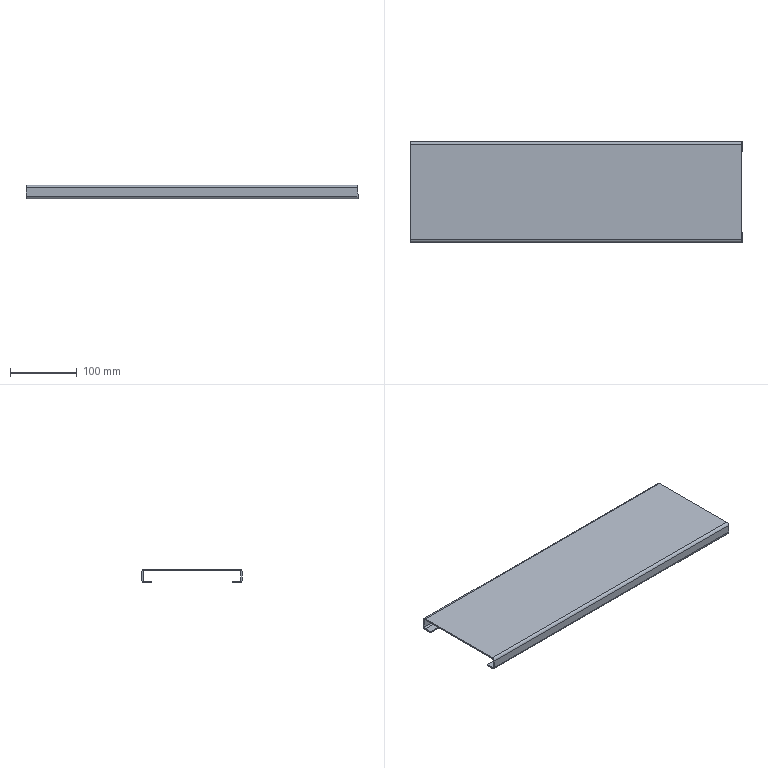Part | SolidWorks | features EdgeFlange 4, Extrusion 1, FlatPattern 1, ICE 1, SheetMetal 1, SolidToSheetMetal 1 | 1 solid | 40 faces | box 496 x 150 x 20 mm | volume 205094 mm3 | plane 30 | cylinder 10 | commonest cylinder face diameters 8 x6 4 x4
STEP:
#1=CARTESIAN_POINT('',(-233.5,73.,-13.));
#2=VERTEX_POINT('',#1);
#3=CARTESIAN_POINT('',(-233.5,73.,-5.));
#4=VERTEX_POINT('',#3);
#5=CARTESIAN_POINT('',(-233.5,73.,-9.));
#6=DIRECTION('',(0.,1.,0.));
#7=DIRECTION('',(0.,0.,1.));
#8=AXIS2_PLACEMENT_3D('',#5,#6,#7);
#9=CIRCLE('',#8,4.);
#10=EDGE_CURVE('',#2,#4,#9,.T.);
#11=ORIENTED_EDGE('',*,*,#10,.F.);
#12=CARTESIAN_POINT('',(-233.5,75.,-13.));
#13=VERTEX_POINT('',#12);
#14=CARTESIAN_POINT('',(-233.5,65.,-13.));
#15=DIRECTION('',(0.,1.,0.));
#16=VECTOR('',#15,1000.);
#17=LINE('',#14,#16);
#18=EDGE_CURVE('',#2,#13,#17,.T.);
#19=ORIENTED_EDGE('',*,*,#18,.T.);
#20=CARTESIAN_POINT('',(-233.5,75.,-5.));
#21=VERTEX_POINT('',#20);
#22=CARTESIAN_POINT('',(-233.5,75.,-9.));
#23=DIRECTION('',(0.,1.,0.));
#24=DIRECTION('',(0.,0.,1.));
#25=AXIS2_PLACEMENT_3D('',#22,#23,#24);
#26=CIRCLE('',#25,4.);
#27=EDGE_CURVE('',#13,#21,#26,.T.);
#28=ORIENTED_EDGE('',*,*,#27,.T.);
#29=CARTESIAN_POINT('',(-233.5,65.,-5.));
#30=DIRECTION('',(0.,1.,0.));
#31=VECTOR('',#30,1000.);
#32=LINE('',#29,#31);
#33=EDGE_CURVE('',#4,#21,#32,.T.);
#34=ORIENTED_EDGE('',*,*,#33,.F.);
#35=EDGE_LOOP('',(#11,#19,#28,#34));
#36=FACE_OUTER_BOUND('',#35,.T.);
#37=CARTESIAN_POINT('',(-233.5,65.,-9.));
#38=DIRECTION('',(0.,1.,0.));
#39=DIRECTION('',(0.,0.,1.));
#40=AXIS2_PLACEMENT_3D('',#37,#38,#39);
#41=CYLINDRICAL_SURFACE('',#40,4.);
#42=ADVANCED_FACE('',(#36),#41,.F.);
#43=CARTESIAN_POINT('',(-248.,-73.,-15.));
#44=VERTEX_POINT('',#43);
#45=CARTESIAN_POINT('',(-248.,-73.,-3.));
#46=VERTEX_POINT('',#45);
#47=CARTESIAN_POINT('',(-248.,-73.,-1.));
#48=DIRECTION('',(0.,0.,1.));
#49=VECTOR('',#48,1000.);
#50=LINE('',#47,#49);
#51=EDGE_CURVE('',#44,#46,#50,.T.);
#52=ORIENTED_EDGE('',*,*,#51,.F.);
#53=CARTESIAN_POINT('',(-248.,-75.,-15.));
#54=VERTEX_POINT('',#53);
#55=CARTESIAN_POINT('',(-248.,-73.,-15.));
#56=DIRECTION('',(0.,-1.,0.));
#57=VECTOR('',#56,1000.);
#58=LINE('',#55,#57);
#59=EDGE_CURVE('',#44,#54,#58,.T.);
#60=ORIENTED_EDGE('',*,*,#59,.T.);
#61=CARTESIAN_POINT('',(-248.,-75.,-3.));
#62=VERTEX_POINT('',#61);
#63=CARTESIAN_POINT('',(-248.,-75.,-1.));
#64=DIRECTION('',(0.,0.,1.));
#65=VECTOR('',#64,1000.);
#66=LINE('',#63,#65);
#67=EDGE_CURVE('',#54,#62,#66,.T.);
#68=ORIENTED_EDGE('',*,*,#67,.T.);
#69=CARTESIAN_POINT('',(-248.,-73.,-3.));
#70=DIRECTION('',(0.,-1.,0.));
#71=VECTOR('',#70,1000.);
#72=LINE('',#69,#71);
#73=EDGE_CURVE('',#46,#62,#72,.T.);
#74=ORIENTED_EDGE('',*,*,#73,.F.);
#75=EDGE_LOOP('',(#52,#60,#68,#74));
#76=FACE_OUTER_BOUND('',#75,.T.);
#77=CARTESIAN_POINT('',(-248.,-75.,-1.));
#78=DIRECTION('',(-1.,0.,0.));
#79=DIRECTION('',(0.,0.,1.));
#80=AXIS2_PLACEMENT_3D('',#77,#78,#79);
#81=PLANE('',#80);
#82=ADVANCED_FACE('',(#76),#81,.T.);
#83=ORIENTED_EDGE('',*,*,#67,.F.);
#84=CARTESIAN_POINT('',(248.,-75.,-15.));
#85=VERTEX_POINT('',#84);
#86=CARTESIAN_POINT('',(-248.,-75.,-15.));
#87=DIRECTION('',(1.,0.,0.));
#88=VECTOR('',#87,1000.);
#89=LINE('',#86,#88);
#90=EDGE_CURVE('',#54,#85,#89,.T.);
#91=ORIENTED_EDGE('',*,*,#90,.T.);
#92=CARTESIAN_POINT('',(248.,-75.,-3.));
#93=VERTEX_POINT('',#92);
#94=CARTESIAN_POINT('',(248.,-75.,-19.));
#95=DIRECTION('',(0.,0.,-1.));
#96=VECTOR('',#95,1000.);
#97=LINE('',#94,#96);
#98=EDGE_CURVE('',#93,#85,#97,.T.);
#99=ORIENTED_EDGE('',*,*,#98,.F.);
#100=CARTESIAN_POINT('',(-248.,-75.,-3.));
#101=DIRECTION('',(-1.,0.,0.));
#102=VECTOR('',#101,1000.);
#103=LINE('',#100,#102);
#104=EDGE_CURVE('',#93,#62,#103,.T.);
#105=ORIENTED_EDGE('',*,*,#104,.T.);
#106=EDGE_LOOP('',(#83,#91,#99,#105));
#107=FACE_OUTER_BOUND('',#106,.T.);
#108=CARTESIAN_POINT('',(-248.,-75.,-1.));
#109=DIRECTION('',(0.,-1.,0.));
#110=DIRECTION('',(0.,0.,-1.));
#111=AXIS2_PLACEMENT_3D('',#108,#109,#110);
#112=PLANE('',#111);
#113=ADVANCED_FACE('',(#107),#112,.T.);
#114=CARTESIAN_POINT('',(248.,-73.,-15.));
#115=VERTEX_POINT('',#114);
#116=CARTESIAN_POINT('',(-248.,-73.,-15.));
#117=DIRECTION('',(1.,0.,0.));
#118=VECTOR('',#117,1000.);
#119=LINE('',#116,#118);
#120=EDGE_CURVE('',#44,#115,#119,.T.);
#121=ORIENTED_EDGE('',*,*,#120,.F.);
#122=ORIENTED_EDGE('',*,*,#51,.T.);
#123=CARTESIAN_POINT('',(248.,-73.,-3.));
#124=VERTEX_POINT('',#123);
#125=CARTESIAN_POINT('',(248.,-73.,-3.));
#126=DIRECTION('',(-1.,0.,0.));
#127=VECTOR('',#126,1000.);
#128=LINE('',#125,#127);
#129=EDGE_CURVE('',#124,#46,#128,.T.);
#130=ORIENTED_EDGE('',*,*,#129,.F.);
#131=CARTESIAN_POINT('',(248.,-73.,-1.));
#132=DIRECTION('',(0.,0.,-1.));
#133=VECTOR('',#132,1000.);
#134=LINE('',#131,#133);
#135=EDGE_CURVE('',#124,#115,#134,.T.);
#136=ORIENTED_EDGE('',*,*,#135,.T.);
#137=EDGE_LOOP('',(#121,#122,#130,#136));
#138=FACE_OUTER_BOUND('',#137,.T.);
#139=CARTESIAN_POINT('',(-248.,-73.,-1.));
#140=DIRECTION('',(0.,-1.,0.));
#141=DIRECTION('',(0.,0.,-1.));
#142=AXIS2_PLACEMENT_3D('',#139,#140,#141);
#143=PLANE('',#142);
#144=ADVANCED_FACE('',(#138),#143,.F.);
#145=CARTESIAN_POINT('',(-248.,71.,1.));
#146=VERTEX_POINT('',#145);
#147=CARTESIAN_POINT('',(-248.,-71.,1.));
#148=VERTEX_POINT('',#147);
#149=CARTESIAN_POINT('',(-248.,75.,1.));
#150=DIRECTION('',(0.,-1.,0.));
#151=VECTOR('',#150,1000.);
#152=LINE('',#149,#151);
#153=EDGE_CURVE('',#146,#148,#152,.T.);
#154=ORIENTED_EDGE('',*,*,#153,.T.);
#155=CARTESIAN_POINT('',(248.,-71.,1.));
#156=VERTEX_POINT('',#155);
#157=CARTESIAN_POINT('',(-248.,-71.,1.));
#158=DIRECTION('',(1.,0.,0.));
#159=VECTOR('',#158,1000.);
#160=LINE('',#157,#159);
#161=EDGE_CURVE('',#148,#156,#160,.T.);
#162=ORIENTED_EDGE('',*,*,#161,.T.);
#163=CARTESIAN_POINT('',(248.,71.,1.));
#164=VERTEX_POINT('',#163);
#165=CARTESIAN_POINT('',(248.,75.,1.));
#166=DIRECTION('',(0.,1.,0.));
#167=VECTOR('',#166,1000.);
#168=LINE('',#165,#167);
#169=EDGE_CURVE('',#156,#164,#168,.T.);
#170=ORIENTED_EDGE('',*,*,#169,.T.);
#171=CARTESIAN_POINT('',(248.,71.,1.));
#172=DIRECTION('',(-1.,0.,0.));
#173=VECTOR('',#172,1000.);
#174=LINE('',#171,#173);
#175=EDGE_CURVE('',#164,#146,#174,.T.);
#176=ORIENTED_EDGE('',*,*,#175,.T.);
#177=EDGE_LOOP('',(#154,#162,#170,#176));
#178=FACE_OUTER_BOUND('',#177,.T.);
#179=CARTESIAN_POINT('',(248.,-75.,1.));
#180=DIRECTION('',(0.,0.,1.));
#181=DIRECTION('',(1.,0.,0.));
#182=AXIS2_PLACEMENT_3D('',#179,#180,#181);
#183=PLANE('',#182);
#184=ADVANCED_FACE('',(#178),#183,.T.);
#185=CARTESIAN_POINT('',(-248.,-71.,-1.));
#186=VERTEX_POINT('',#185);
#187=CARTESIAN_POINT('',(248.,-71.,-1.));
#188=VERTEX_POINT('',#187);
#189=CARTESIAN_POINT('',(-248.,-71.,-1.));
#190=DIRECTION('',(1.,0.,0.));
#191=VECTOR('',#190,1000.);
#192=LINE('',#189,#191);
#193=EDGE_CURVE('',#186,#188,#192,.T.);
#194=ORIENTED_EDGE('',*,*,#193,.F.);
#195=CARTESIAN_POINT('',(-248.,71.,-1.));
#196=VERTEX_POINT('',#195);
#197=CARTESIAN_POINT('',(-248.,-75.,-1.));
#198=DIRECTION('',(0.,-1.,0.));
#199=VECTOR('',#198,1000.);
#200=LINE('',#197,#199);
#201=EDGE_CURVE('',#196,#186,#200,.T.);
#202=ORIENTED_EDGE('',*,*,#201,.F.);
#203=CARTESIAN_POINT('',(248.,71.,-1.));
#204=VERTEX_POINT('',#203);
#205=CARTESIAN_POINT('',(248.,71.,-1.));
#206=DIRECTION('',(-1.,0.,0.));
#207=VECTOR('',#206,1000.);
#208=LINE('',#205,#207);
#209=EDGE_CURVE('',#204,#196,#208,.T.);
#210=ORIENTED_EDGE('',*,*,#209,.F.);
#211=CARTESIAN_POINT('',(248.,-75.,-1.));
#212=DIRECTION('',(0.,1.,0.));
#213=VECTOR('',#212,1000.);
#214=LINE('',#211,#213);
#215=EDGE_CURVE('',#188,#204,#214,.T.);
#216=ORIENTED_EDGE('',*,*,#215,.F.);
#217=EDGE_LOOP('',(#194,#202,#210,#216));
#218=FACE_OUTER_BOUND('',#217,.T.);
#219=CARTESIAN_POINT('',(248.,-75.,-1.));
#220=DIRECTION('',(0.,0.,1.));
#221=DIRECTION('',(1.,0.,0.));
#222=AXIS2_PLACEMENT_3D('',#219,#220,#221);
#223=PLANE('',#222);
#224=ADVANCED_FACE('',(#218),#223,.F.);
#225=ORIENTED_EDGE('',*,*,#201,.T.);
#226=CARTESIAN_POINT('',(-248.,-71.,-1.));
#227=DIRECTION('',(0.,0.,1.));
#228=VECTOR('',#227,1000.);
#229=LINE('',#226,#228);
#230=EDGE_CURVE('',#186,#148,#229,.T.);
#231=ORIENTED_EDGE('',*,*,#230,.T.);
#232=ORIENTED_EDGE('',*,*,#153,.F.);
#233=CARTESIAN_POINT('',(-248.,71.,-1.));
#234=DIRECTION('',(0.,0.,1.));
#235=VECTOR('',#234,1000.);
#236=LINE('',#233,#235);
#237=EDGE_CURVE('',#196,#146,#236,.T.);
#238=ORIENTED_EDGE('',*,*,#237,.F.);
#239=EDGE_LOOP('',(#225,#231,#232,#238));
#240=FACE_OUTER_BOUND('',#239,.T.);
#241=CARTESIAN_POINT('',(-248.,75.,1.));
#242=DIRECTION('',(-1.,0.,0.));
#243=DIRECTION('',(0.,-1.,0.));
#244=AXIS2_PLACEMENT_3D('',#241,#242,#243);
#245=PLANE('',#244);
#246=ADVANCED_FACE('',(#240),#245,.T.);
#247=CARTESIAN_POINT('',(248.,73.,-15.));
#248=VERTEX_POINT('',#247);
#249=CARTESIAN_POINT('',(248.,73.,-3.));
#250=VERTEX_POINT('',#249);
#251=CARTESIAN_POINT('',(248.,73.,-1.));
#252=DIRECTION('',(0.,0.,1.));
#253=VECTOR('',#252,1000.);
#254=LINE('',#251,#253);
#255=EDGE_CURVE('',#248,#250,#254,.T.);
#256=ORIENTED_EDGE('',*,*,#255,.F.);
#257=CARTESIAN_POINT('',(248.,75.,-15.));
#258=VERTEX_POINT('',#257);
#259=CARTESIAN_POINT('',(248.,73.,-15.));
#260=DIRECTION('',(0.,1.,0.));
#261=VECTOR('',#260,1000.);
#262=LINE('',#259,#261);
#263=EDGE_CURVE('',#248,#258,#262,.T.);
#264=ORIENTED_EDGE('',*,*,#263,.T.);
#265=CARTESIAN_POINT('',(248.,75.,-3.));
#266=VERTEX_POINT('',#265);
#267=CARTESIAN_POINT('',(248.,75.,-1.));
#268=DIRECTION('',(0.,0.,1.));
#269=VECTOR('',#268,1000.);
#270=LINE('',#267,#269);
#271=EDGE_CURVE('',#258,#266,#270,.T.);
#272=ORIENTED_EDGE('',*,*,#271,.T.);
#273=CARTESIAN_POINT('',(248.,73.,-3.));
#274=DIRECTION('',(0.,1.,0.));
#275=VECTOR('',#274,1000.);
#276=LINE('',#273,#275);
#277=EDGE_CURVE('',#250,#266,#276,.T.);
#278=ORIENTED_EDGE('',*,*,#277,.F.);
#279=EDGE_LOOP('',(#256,#264,#272,#278));
#280=FACE_OUTER_BOUND('',#279,.T.);
#281=CARTESIAN_POINT('',(248.,75.,-1.));
#282=DIRECTION('',(1.,0.,0.));
#283=DIRECTION('',(0.,0.,-1.));
#284=AXIS2_PLACEMENT_3D('',#281,#282,#283);
#285=PLANE('',#284);
#286=ADVANCED_FACE('',(#280),#285,.T.);
#287=CARTESIAN_POINT('',(-233.5,75.,-9.));
#288=DIRECTION('',(0.,1.,0.));
#289=DIRECTION('',(0.,0.,1.));
#290=AXIS2_PLACEMENT_3D('',#287,#288,#289);
#291=CIRCLE('',#290,4.);
#292=EDGE_CURVE('',#21,#13,#291,.T.);
#293=ORIENTED_EDGE('',*,*,#292,.F.);
#294=ORIENTED_EDGE('',*,*,#27,.F.);
#295=EDGE_LOOP('',(#293,#294));
#296=FACE_BOUND('',#295,.T.);
#297=ORIENTED_EDGE('',*,*,#271,.F.);
#298=CARTESIAN_POINT('',(-248.,75.,-15.));
#299=VERTEX_POINT('',#298);
#300=CARTESIAN_POINT('',(248.,75.,-15.));
#301=DIRECTION('',(-1.,0.,0.));
#302=VECTOR('',#301,1000.);
#303=LINE('',#300,#302);
#304=EDGE_CURVE('',#258,#299,#303,.T.);
#305=ORIENTED_EDGE('',*,*,#304,.T.);
#306=CARTESIAN_POINT('',(-248.,75.,-3.));
#307=VERTEX_POINT('',#306);
#308=CARTESIAN_POINT('',(-248.,75.,-19.));
#309=DIRECTION('',(0.,0.,-1.));
#310=VECTOR('',#309,1000.);
#311=LINE('',#308,#310);
#312=EDGE_CURVE('',#307,#299,#311,.T.);
#313=ORIENTED_EDGE('',*,*,#312,.F.);
#314=CARTESIAN_POINT('',(248.,75.,-3.));
#315=DIRECTION('',(1.,0.,0.));
#316=VECTOR('',#315,1000.);
#317=LINE('',#314,#316);
#318=EDGE_CURVE('',#307,#266,#317,.T.);
#319=ORIENTED_EDGE('',*,*,#318,.T.);
#320=EDGE_LOOP('',(#297,#305,#313,#319));
#321=FACE_OUTER_BOUND('',#320,.T.);
#322=CARTESIAN_POINT('',(248.,75.,-1.));
#323=DIRECTION('',(0.,1.,0.));
#324=DIRECTION('',(0.,0.,1.));
#325=AXIS2_PLACEMENT_3D('',#322,#323,#324);
#326=PLANE('',#325);
#327=ADVANCED_FACE('',(#296,#321),#326,.T.);
#328=CARTESIAN_POINT('',(-233.5,73.,-9.));
#329=DIRECTION('',(0.,1.,0.));
#330=DIRECTION('',(0.,0.,1.));
#331=AXIS2_PLACEMENT_3D('',#328,#329,#330);
#332=CIRCLE('',#331,4.);
#333=EDGE_CURVE('',#4,#2,#332,.T.);
#334=ORIENTED_EDGE('',*,*,#333,.T.);
#335=ORIENTED_EDGE('',*,*,#10,.T.);
#336=EDGE_LOOP('',(#334,#335));
#337=FACE_BOUND('',#336,.T.);
#338=CARTESIAN_POINT('',(-248.,73.,-15.));
#339=VERTEX_POINT('',#338);
#340=CARTESIAN_POINT('',(248.,73.,-15.));
#341=DIRECTION('',(-1.,0.,0.));
#342=VECTOR('',#341,1000.);
#343=LINE('',#340,#342);
#344=EDGE_CURVE('',#248,#339,#343,.T.);
#345=ORIENTED_EDGE('',*,*,#344,.F.);
#346=ORIENTED_EDGE('',*,*,#255,.T.);
#347=CARTESIAN_POINT('',(-248.,73.,-3.));
#348=VERTEX_POINT('',#347);
#349=CARTESIAN_POINT('',(-248.,73.,-3.));
#350=DIRECTION('',(1.,0.,0.));
#351=VECTOR('',#350,1000.);
#352=LINE('',#349,#351);
#353=EDGE_CURVE('',#348,#250,#352,.T.);
#354=ORIENTED_EDGE('',*,*,#353,.F.);
#355=CARTESIAN_POINT('',(-248.,73.,-1.));
#356=DIRECTION('',(0.,0.,-1.));
#357=VECTOR('',#356,1000.);
#358=LINE('',#355,#357);
#359=EDGE_CURVE('',#348,#339,#358,.T.);
#360=ORIENTED_EDGE('',*,*,#359,.T.);
#361=EDGE_LOOP('',(#345,#346,#354,#360));
#362=FACE_OUTER_BOUND('',#361,.T.);
#363=CARTESIAN_POINT('',(248.,73.,-1.));
#364=DIRECTION('',(0.,1.,0.));
#365=DIRECTION('',(0.,0.,1.));
#366=AXIS2_PLACEMENT_3D('',#363,#364,#365);
#367=PLANE('',#366);
#368=ADVANCED_FACE('',(#337,#362),#367,.F.);
#369=CARTESIAN_POINT('',(248.,-71.,-1.));
#370=DIRECTION('',(0.,0.,1.));
#371=VECTOR('',#370,1000.);
#372=LINE('',#369,#371);
#373=EDGE_CURVE('',#188,#156,#372,.T.);
#374=ORIENTED_EDGE('',*,*,#373,.F.);
#375=ORIENTED_EDGE('',*,*,#215,.T.);
#376=CARTESIAN_POINT('',(248.,71.,-1.));
#377=DIRECTION('',(0.,0.,1.));
#378=VECTOR('',#377,1000.);
#379=LINE('',#376,#378);
#380=EDGE_CURVE('',#204,#164,#379,.T.);
#381=ORIENTED_EDGE('',*,*,#380,.T.);
#382=ORIENTED_EDGE('',*,*,#169,.F.);
#383=EDGE_LOOP('',(#374,#375,#381,#382));
#384=FACE_OUTER_BOUND('',#383,.T.);
#385=CARTESIAN_POINT('',(248.,75.,1.));
#386=DIRECTION('',(1.,0.,0.));
#387=DIRECTION('',(0.,1.,0.));
#388=AXIS2_PLACEMENT_3D('',#385,#386,#387);
#389=PLANE('',#388);
#390=ADVANCED_FACE('',(#384),#389,.T.);
#391=CARTESIAN_POINT('',(-248.,75.,-3.));
#392=DIRECTION('',(0.,1.,0.));
#393=VECTOR('',#392,1000.);
#394=LINE('',#391,#393);
#395=EDGE_CURVE('',#348,#307,#394,.T.);
#396=ORIENTED_EDGE('',*,*,#395,.F.);
#397=CARTESIAN_POINT('',(-248.,71.,-3.));
#398=DIRECTION('',(-1.,0.,0.));
#399=DIRECTION('',(0.,0.,-1.));
#400=AXIS2_PLACEMENT_3D('',#397,#398,#399);
#401=CIRCLE('',#400,2.);
#402=EDGE_CURVE('',#196,#348,#401,.T.);
#403=ORIENTED_EDGE('',*,*,#402,.F.);
#404=ORIENTED_EDGE('',*,*,#237,.T.);
#405=CARTESIAN_POINT('',(-248.,71.,-3.));
#406=DIRECTION('',(-1.,0.,0.));
#407=DIRECTION('',(0.,0.,-1.));
#408=AXIS2_PLACEMENT_3D('',#405,#406,#407);
#409=CIRCLE('',#408,4.);
#410=EDGE_CURVE('',#146,#307,#409,.T.);
#411=ORIENTED_EDGE('',*,*,#410,.T.);
#412=EDGE_LOOP('',(#396,#403,#404,#411));
#413=FACE_OUTER_BOUND('',#412,.T.);
#414=CARTESIAN_POINT('',(-248.,71.,-3.));
#415=DIRECTION('',(-1.,0.,0.));
#416=DIRECTION('',(0.,0.,1.));
#417=AXIS2_PLACEMENT_3D('',#414,#415,#416);
#418=PLANE('',#417);
#419=ADVANCED_FACE('',(#413),#418,.T.);
#420=ORIENTED_EDGE('',*,*,#175,.F.);
#421=CARTESIAN_POINT('',(248.,71.,-3.));
#422=DIRECTION('',(1.,0.,0.));
#423=DIRECTION('',(0.,0.,-1.));
#424=AXIS2_PLACEMENT_3D('',#421,#422,#423);
#425=CIRCLE('',#424,4.);
#426=EDGE_CURVE('',#266,#164,#425,.T.);
#427=ORIENTED_EDGE('',*,*,#426,.F.);
#428=ORIENTED_EDGE('',*,*,#318,.F.);
#429=ORIENTED_EDGE('',*,*,#410,.F.);
#430=EDGE_LOOP('',(#420,#427,#428,#429));
#431=FACE_OUTER_BOUND('',#430,.T.);
#432=CARTESIAN_POINT('',(248.,71.,-3.));
#433=DIRECTION('',(1.,0.,0.));
#434=DIRECTION('',(0.,1.,0.));
#435=AXIS2_PLACEMENT_3D('',#432,#433,#434);
#436=CYLINDRICAL_SURFACE('',#435,4.);
#437=ADVANCED_FACE('',(#431),#436,.T.);
#438=CARTESIAN_POINT('',(248.,71.,-3.));
#439=DIRECTION('',(1.,0.,0.));
#440=DIRECTION('',(0.,0.,-1.));
#441=AXIS2_PLACEMENT_3D('',#438,#439,#440);
#442=CIRCLE('',#441,2.);
#443=EDGE_CURVE('',#250,#204,#442,.T.);
#444=ORIENTED_EDGE('',*,*,#443,.F.);
#445=ORIENTED_EDGE('',*,*,#277,.T.);
#446=ORIENTED_EDGE('',*,*,#426,.T.);
#447=ORIENTED_EDGE('',*,*,#380,.F.);
#448=EDGE_LOOP('',(#444,#445,#446,#447));
#449=FACE_OUTER_BOUND('',#448,.T.);
#450=CARTESIAN_POINT('',(248.,71.,-3.));
#451=DIRECTION('',(-1.,0.,0.));
#452=DIRECTION('',(0.,0.,1.));
#453=AXIS2_PLACEMENT_3D('',#450,#451,#452);
#454=PLANE('',#453);
#455=ADVANCED_FACE('',(#449),#454,.F.);
#456=ORIENTED_EDGE('',*,*,#209,.T.);
#457=ORIENTED_EDGE('',*,*,#402,.T.);
#458=ORIENTED_EDGE('',*,*,#353,.T.);
#459=ORIENTED_EDGE('',*,*,#443,.T.);
#460=EDGE_LOOP('',(#456,#457,#458,#459));
#461=FACE_OUTER_BOUND('',#460,.T.);
#462=CARTESIAN_POINT('',(248.,71.,-3.));
#463=DIRECTION('',(1.,0.,0.));
#464=DIRECTION('',(0.,1.,0.));
#465=AXIS2_PLACEMENT_3D('',#462,#463,#464);
#466=CYLINDRICAL_SURFACE('',#465,2.);
#467=ADVANCED_FACE('',(#461),#466,.F.);
#468=CARTESIAN_POINT('',(-248.,73.,-15.));
#469=DIRECTION('',(0.,1.,0.));
#470=VECTOR('',#469,1000.);
#471=LINE('',#468,#470);
#472=EDGE_CURVE('',#339,#299,#471,.T.);
#473=ORIENTED_EDGE('',*,*,#472,.F.);
#474=ORIENTED_EDGE('',*,*,#359,.F.);
#475=ORIENTED_EDGE('',*,*,#395,.T.);
#476=ORIENTED_EDGE('',*,*,#312,.T.);
#477=EDGE_LOOP('',(#473,#474,#475,#476));
#478=FACE_OUTER_BOUND('',#477,.T.);
#479=CARTESIAN_POINT('',(-248.,75.,-19.));
#480=DIRECTION('',(-1.,0.,0.));
#481=DIRECTION('',(0.,0.,1.));
#482=AXIS2_PLACEMENT_3D('',#479,#480,#481);
#483=PLANE('',#482);
#484=ADVANCED_FACE('',(#478),#483,.T.);
#485=CARTESIAN_POINT('',(-248.,71.,-17.));
#486=VERTEX_POINT('',#485);
#487=CARTESIAN_POINT('',(-248.,71.,-19.));
#488=VERTEX_POINT('',#487);
#489=CARTESIAN_POINT('',(-248.,71.,-19.));
#490=DIRECTION('',(0.,0.,-1.));
#491=VECTOR('',#490,1000.);
#492=LINE('',#489,#491);
#493=EDGE_CURVE('',#486,#488,#492,.T.);
#494=ORIENTED_EDGE('',*,*,#493,.F.);
#495=CARTESIAN_POINT('',(-248.,71.,-15.));
#496=DIRECTION('',(-1.,0.,0.));
#497=DIRECTION('',(0.,0.,-1.));
#498=AXIS2_PLACEMENT_3D('',#495,#496,#497);
#499=CIRCLE('',#498,2.);
#500=EDGE_CURVE('',#339,#486,#499,.T.);
#501=ORIENTED_EDGE('',*,*,#500,.F.);
#502=ORIENTED_EDGE('',*,*,#472,.T.);
#503=CARTESIAN_POINT('',(-248.,71.,-15.));
#504=DIRECTION('',(-1.,0.,0.));
#505=DIRECTION('',(0.,0.,-1.));
#506=AXIS2_PLACEMENT_3D('',#503,#504,#505);
#507=CIRCLE('',#506,4.);
#508=EDGE_CURVE('',#299,#488,#507,.T.);
#509=ORIENTED_EDGE('',*,*,#508,.T.);
#510=EDGE_LOOP('',(#494,#501,#502,#509));
#511=FACE_OUTER_BOUND('',#510,.T.);
#512=CARTESIAN_POINT('',(-248.,71.,-15.));
#513=DIRECTION('',(-1.,0.,0.));
#514=DIRECTION('',(0.,0.,1.));
#515=AXIS2_PLACEMENT_3D('',#512,#513,#514);
#516=PLANE('',#515);
#517=ADVANCED_FACE('',(#511),#516,.T.);
#518=ORIENTED_EDGE('',*,*,#304,.F.);
#519=CARTESIAN_POINT('',(248.,71.,-19.));
#520=VERTEX_POINT('',#519);
#521=CARTESIAN_POINT('',(248.,71.,-15.));
#522=DIRECTION('',(1.,0.,0.));
#523=DIRECTION('',(0.,0.,-1.));
#524=AXIS2_PLACEMENT_3D('',#521,#522,#523);
#525=CIRCLE('',#524,4.);
#526=EDGE_CURVE('',#520,#258,#525,.T.);
#527=ORIENTED_EDGE('',*,*,#526,.F.);
#528=CARTESIAN_POINT('',(248.,71.,-19.));
#529=DIRECTION('',(1.,0.,0.));
#530=VECTOR('',#529,1000.);
#531=LINE('',#528,#530);
#532=EDGE_CURVE('',#488,#520,#531,.T.);
#533=ORIENTED_EDGE('',*,*,#532,.F.);
#534=ORIENTED_EDGE('',*,*,#508,.F.);
#535=EDGE_LOOP('',(#518,#527,#533,#534));
#536=FACE_OUTER_BOUND('',#535,.T.);
#537=CARTESIAN_POINT('',(248.,71.,-15.));
#538=DIRECTION('',(1.,0.,0.));
#539=DIRECTION('',(0.,0.,-1.));
#540=AXIS2_PLACEMENT_3D('',#537,#538,#539);
#541=CYLINDRICAL_SURFACE('',#540,4.);
#542=ADVANCED_FACE('',(#536),#541,.T.);
#543=CARTESIAN_POINT('',(248.,71.,-17.));
#544=VERTEX_POINT('',#543);
#545=CARTESIAN_POINT('',(248.,71.,-15.));
#546=DIRECTION('',(1.,0.,0.));
#547=DIRECTION('',(0.,0.,-1.));
#548=AXIS2_PLACEMENT_3D('',#545,#546,#547);
#549=CIRCLE('',#548,2.);
#550=EDGE_CURVE('',#544,#248,#549,.T.);
#551=ORIENTED_EDGE('',*,*,#550,.F.);
#552=CARTESIAN_POINT('',(248.,71.,-17.));
#553=DIRECTION('',(0.,0.,-1.));
#554=VECTOR('',#553,1000.);
#555=LINE('',#552,#554);
#556=EDGE_CURVE('',#544,#520,#555,.T.);
#557=ORIENTED_EDGE('',*,*,#556,.T.);
#558=ORIENTED_EDGE('',*,*,#526,.T.);
#559=ORIENTED_EDGE('',*,*,#263,.F.);
#560=EDGE_LOOP('',(#551,#557,#558,#559));
#561=FACE_OUTER_BOUND('',#560,.T.);
#562=CARTESIAN_POINT('',(248.,71.,-15.));
#563=DIRECTION('',(-1.,0.,0.));
#564=DIRECTION('',(0.,0.,1.));
#565=AXIS2_PLACEMENT_3D('',#562,#563,#564);
#566=PLANE('',#565);
#567=ADVANCED_FACE('',(#561),#566,.F.);
#568=ORIENTED_EDGE('',*,*,#344,.T.);
#569=ORIENTED_EDGE('',*,*,#500,.T.);
#570=CARTESIAN_POINT('',(-248.,71.,-17.));
#571=DIRECTION('',(1.,0.,0.));
#572=VECTOR('',#571,1000.);
#573=LINE('',#570,#572);
#574=EDGE_CURVE('',#486,#544,#573,.T.);
#575=ORIENTED_EDGE('',*,*,#574,.T.);
#576=ORIENTED_EDGE('',*,*,#550,.T.);
#577=EDGE_LOOP('',(#568,#569,#575,#576));
#578=FACE_OUTER_BOUND('',#577,.T.);
#579=CARTESIAN_POINT('',(248.,71.,-15.));
#580=DIRECTION('',(1.,0.,0.));
#581=DIRECTION('',(0.,0.,-1.));
#582=AXIS2_PLACEMENT_3D('',#579,#580,#581);
#583=CYLINDRICAL_SURFACE('',#582,2.);
#584=ADVANCED_FACE('',(#578),#583,.F.);
#585=CARTESIAN_POINT('',(248.,60.,-19.));
#586=VERTEX_POINT('',#585);
#587=CARTESIAN_POINT('',(248.,73.,-19.));
#588=DIRECTION('',(0.,1.,0.));
#589=VECTOR('',#588,1000.);
#590=LINE('',#587,#589);
#591=EDGE_CURVE('',#586,#520,#590,.T.);
#592=ORIENTED_EDGE('',*,*,#591,.T.);
#593=ORIENTED_EDGE('',*,*,#556,.F.);
#594=CARTESIAN_POINT('',(248.,60.,-17.));
#595=VERTEX_POINT('',#594);
#596=CARTESIAN_POINT('',(248.,73.,-17.));
#597=DIRECTION('',(0.,1.,0.));
#598=VECTOR('',#597,1000.);
#599=LINE('',#596,#598);
#600=EDGE_CURVE('',#595,#544,#599,.T.);
#601=ORIENTED_EDGE('',*,*,#600,.F.);
#602=CARTESIAN_POINT('',(248.,60.,-19.));
#603=DIRECTION('',(0.,0.,1.));
#604=VECTOR('',#603,1000.);
#605=LINE('',#602,#604);
#606=EDGE_CURVE('',#586,#595,#605,.T.);
#607=ORIENTED_EDGE('',*,*,#606,.F.);
#608=EDGE_LOOP('',(#592,#593,#601,#607));
#609=FACE_OUTER_BOUND('',#608,.T.);
#610=CARTESIAN_POINT('',(248.,73.,-19.));
#611=DIRECTION('',(1.,0.,0.));
#612=DIRECTION('',(0.,0.,-1.));
#613=AXIS2_PLACEMENT_3D('',#610,#611,#612);
#614=PLANE('',#613);
#615=ADVANCED_FACE('',(#609),#614,.T.);
#616=CARTESIAN_POINT('',(-248.,60.,-17.));
#617=VERTEX_POINT('',#616);
#618=CARTESIAN_POINT('',(-248.,73.,-17.));
#619=DIRECTION('',(0.,-1.,0.));
#620=VECTOR('',#619,1000.);
#621=LINE('',#618,#620);
#622=EDGE_CURVE('',#486,#617,#621,.T.);
#623=ORIENTED_EDGE('',*,*,#622,.F.);
#624=ORIENTED_EDGE('',*,*,#493,.T.);
#625=CARTESIAN_POINT('',(-248.,60.,-19.));
#626=VERTEX_POINT('',#625);
#627=CARTESIAN_POINT('',(-248.,60.,-19.));
#628=DIRECTION('',(0.,-1.,0.));
#629=VECTOR('',#628,1000.);
#630=LINE('',#627,#629);
#631=EDGE_CURVE('',#488,#626,#630,.T.);
#632=ORIENTED_EDGE('',*,*,#631,.T.);
#633=CARTESIAN_POINT('',(-248.,60.,-19.));
#634=DIRECTION('',(0.,0.,1.));
#635=VECTOR('',#634,1000.);
#636=LINE('',#633,#635);
#637=EDGE_CURVE('',#626,#617,#636,.T.);
#638=ORIENTED_EDGE('',*,*,#637,.T.);
#639=EDGE_LOOP('',(#623,#624,#632,#638));
#640=FACE_OUTER_BOUND('',#639,.T.);
#641=CARTESIAN_POINT('',(-248.,60.,-19.));
#642=DIRECTION('',(-1.,0.,0.));
#643=DIRECTION('',(0.,0.,1.));
#644=AXIS2_PLACEMENT_3D('',#641,#642,#643);
#645=PLANE('',#644);
#646=ADVANCED_FACE('',(#640),#645,.T.);
#647=ORIENTED_EDGE('',*,*,#631,.F.);
#648=ORIENTED_EDGE('',*,*,#532,.T.);
#649=ORIENTED_EDGE('',*,*,#591,.F.);
#650=CARTESIAN_POINT('',(248.,60.,-19.));
#651=DIRECTION('',(1.,0.,0.));
#652=VECTOR('',#651,1000.);
#653=LINE('',#650,#652);
#654=EDGE_CURVE('',#626,#586,#653,.T.);
#655=ORIENTED_EDGE('',*,*,#654,.F.);
#656=EDGE_LOOP('',(#647,#648,#649,#655));
#657=FACE_OUTER_BOUND('',#656,.T.);
#658=CARTESIAN_POINT('',(248.,73.,-19.));
#659=DIRECTION('',(0.,0.,-1.));
#660=DIRECTION('',(0.,1.,0.));
#661=AXIS2_PLACEMENT_3D('',#658,#659,#660);
#662=PLANE('',#661);
#663=ADVANCED_FACE('',(#657),#662,.T.);
#664=ORIENTED_EDGE('',*,*,#574,.F.);
#665=ORIENTED_EDGE('',*,*,#622,.T.);
#666=CARTESIAN_POINT('',(248.,60.,-17.));
#667=DIRECTION('',(1.,0.,0.));
#668=VECTOR('',#667,1000.);
#669=LINE('',#666,#668);
#670=EDGE_CURVE('',#617,#595,#669,.T.);
#671=ORIENTED_EDGE('',*,*,#670,.T.);
#672=ORIENTED_EDGE('',*,*,#600,.T.);
#673=EDGE_LOOP('',(#664,#665,#671,#672));
#674=FACE_OUTER_BOUND('',#673,.T.);
#675=CARTESIAN_POINT('',(248.,73.,-17.));
#676=DIRECTION('',(0.,0.,-1.));
#677=DIRECTION('',(0.,1.,0.));
#678=AXIS2_PLACEMENT_3D('',#675,#676,#677);
#679=PLANE('',#678);
#680=ADVANCED_FACE('',(#674),#679,.F.);
#681=ORIENTED_EDGE('',*,*,#670,.F.);
#682=ORIENTED_EDGE('',*,*,#637,.F.);
#683=ORIENTED_EDGE('',*,*,#654,.T.);
#684=ORIENTED_EDGE('',*,*,#606,.T.);
#685=EDGE_LOOP('',(#681,#682,#683,#684));
#686=FACE_OUTER_BOUND('',#685,.T.);
#687=CARTESIAN_POINT('',(248.,60.,-19.));
#688=DIRECTION('',(0.,-1.,0.));
#689=DIRECTION('',(0.,0.,-1.));
#690=AXIS2_PLACEMENT_3D('',#687,#688,#689);
#691=PLANE('',#690);
#692=ADVANCED_FACE('',(#686),#691,.T.);
#693=CARTESIAN_POINT('',(248.,-75.,-3.));
#694=DIRECTION('',(0.,-1.,0.));
#695=VECTOR('',#694,1000.);
#696=LINE('',#693,#695);
#697=EDGE_CURVE('',#124,#93,#696,.T.);
#698=ORIENTED_EDGE('',*,*,#697,.F.);
#699=CARTESIAN_POINT('',(248.,-71.,-3.));
#700=DIRECTION('',(1.,0.,0.));
#701=DIRECTION('',(0.,0.,1.));
#702=AXIS2_PLACEMENT_3D('',#699,#700,#701);
#703=CIRCLE('',#702,2.);
#704=EDGE_CURVE('',#188,#124,#703,.T.);
#705=ORIENTED_EDGE('',*,*,#704,.F.);
#706=ORIENTED_EDGE('',*,*,#373,.T.);
#707=CARTESIAN_POINT('',(248.,-71.,-3.));
#708=DIRECTION('',(1.,0.,0.));
#709=DIRECTION('',(0.,0.,1.));
#710=AXIS2_PLACEMENT_3D('',#707,#708,#709);
#711=CIRCLE('',#710,4.);
#712=EDGE_CURVE('',#156,#93,#711,.T.);
#713=ORIENTED_EDGE('',*,*,#712,.T.);
#714=EDGE_LOOP('',(#698,#705,#706,#713));
#715=FACE_OUTER_BOUND('',#714,.T.);
#716=CARTESIAN_POINT('',(248.,-71.,-3.));
#717=DIRECTION('',(1.,0.,0.));
#718=DIRECTION('',(0.,0.,-1.));
#719=AXIS2_PLACEMENT_3D('',#716,#717,#718);
#720=PLANE('',#719);
#721=ADVANCED_FACE('',(#715),#720,.T.);
#722=ORIENTED_EDGE('',*,*,#161,.F.);
#723=CARTESIAN_POINT('',(-248.,-71.,-3.));
#724=DIRECTION('',(-1.,0.,0.));
#725=DIRECTION('',(0.,0.,1.));
#726=AXIS2_PLACEMENT_3D('',#723,#724,#725);
#727=CIRCLE('',#726,4.);
#728=EDGE_CURVE('',#62,#148,#727,.T.);
#729=ORIENTED_EDGE('',*,*,#728,.F.);
#730=ORIENTED_EDGE('',*,*,#104,.F.);
#731=ORIENTED_EDGE('',*,*,#712,.F.);
#732=EDGE_LOOP('',(#722,#729,#730,#731));
#733=FACE_OUTER_BOUND('',#732,.T.);
#734=CARTESIAN_POINT('',(-248.,-71.,-3.));
#735=DIRECTION('',(-1.,0.,0.));
#736=DIRECTION('',(0.,-1.,0.));
#737=AXIS2_PLACEMENT_3D('',#734,#735,#736);
#738=CYLINDRICAL_SURFACE('',#737,4.);
#739=ADVANCED_FACE('',(#733),#738,.T.);
#740=CARTESIAN_POINT('',(-248.,-71.,-3.));
#741=DIRECTION('',(-1.,0.,0.));
#742=DIRECTION('',(0.,0.,1.));
#743=AXIS2_PLACEMENT_3D('',#740,#741,#742);
#744=CIRCLE('',#743,2.);
#745=EDGE_CURVE('',#46,#186,#744,.T.);
#746=ORIENTED_EDGE('',*,*,#745,.F.);
#747=ORIENTED_EDGE('',*,*,#73,.T.);
#748=ORIENTED_EDGE('',*,*,#728,.T.);
#749=ORIENTED_EDGE('',*,*,#230,.F.);
#750=EDGE_LOOP('',(#746,#747,#748,#749));
#751=FACE_OUTER_BOUND('',#750,.T.);
#752=CARTESIAN_POINT('',(-248.,-71.,-3.));
#753=DIRECTION('',(1.,0.,0.));
#754=DIRECTION('',(0.,0.,-1.));
#755=AXIS2_PLACEMENT_3D('',#752,#753,#754);
#756=PLANE('',#755);
#757=ADVANCED_FACE('',(#751),#756,.F.);
#758=ORIENTED_EDGE('',*,*,#193,.T.);
#759=ORIENTED_EDGE('',*,*,#704,.T.);
#760=ORIENTED_EDGE('',*,*,#129,.T.);
#761=ORIENTED_EDGE('',*,*,#745,.T.);
#762=EDGE_LOOP('',(#758,#759,#760,#761));
#763=FACE_OUTER_BOUND('',#762,.T.);
#764=CARTESIAN_POINT('',(-248.,-71.,-3.));
#765=DIRECTION('',(-1.,0.,0.));
#766=DIRECTION('',(0.,-1.,0.));
#767=AXIS2_PLACEMENT_3D('',#764,#765,#766);
#768=CYLINDRICAL_SURFACE('',#767,2.);
#769=ADVANCED_FACE('',(#763),#768,.F.);
#770=CARTESIAN_POINT('',(248.,-73.,-15.));
#771=DIRECTION('',(0.,-1.,0.));
#772=VECTOR('',#771,1000.);
#773=LINE('',#770,#772);
#774=EDGE_CURVE('',#115,#85,#773,.T.);
#775=ORIENTED_EDGE('',*,*,#774,.F.);
#776=ORIENTED_EDGE('',*,*,#135,.F.);
#777=ORIENTED_EDGE('',*,*,#697,.T.);
#778=ORIENTED_EDGE('',*,*,#98,.T.);
#779=EDGE_LOOP('',(#775,#776,#777,#778));
#780=FACE_OUTER_BOUND('',#779,.T.);
#781=CARTESIAN_POINT('',(248.,-75.,-19.));
#782=DIRECTION('',(1.,0.,0.));
#783=DIRECTION('',(0.,0.,-1.));
#784=AXIS2_PLACEMENT_3D('',#781,#782,#783);
#785=PLANE('',#784);
#786=ADVANCED_FACE('',(#780),#785,.T.);
#787=CARTESIAN_POINT('',(248.,-71.,-17.));
#788=VERTEX_POINT('',#787);
#789=CARTESIAN_POINT('',(248.,-71.,-19.));
#790=VERTEX_POINT('',#789);
#791=CARTESIAN_POINT('',(248.,-71.,-19.));
#792=DIRECTION('',(0.,0.,-1.));
#793=VECTOR('',#792,1000.);
#794=LINE('',#791,#793);
#795=EDGE_CURVE('',#788,#790,#794,.T.);
#796=ORIENTED_EDGE('',*,*,#795,.F.);
#797=CARTESIAN_POINT('',(248.,-71.,-15.));
#798=DIRECTION('',(1.,0.,0.));
#799=DIRECTION('',(0.,0.,1.));
#800=AXIS2_PLACEMENT_3D('',#797,#798,#799);
#801=CIRCLE('',#800,2.);
#802=EDGE_CURVE('',#115,#788,#801,.T.);
#803=ORIENTED_EDGE('',*,*,#802,.F.);
#804=ORIENTED_EDGE('',*,*,#774,.T.);
#805=CARTESIAN_POINT('',(248.,-71.,-15.));
#806=DIRECTION('',(1.,0.,0.));
#807=DIRECTION('',(0.,0.,1.));
#808=AXIS2_PLACEMENT_3D('',#805,#806,#807);
#809=CIRCLE('',#808,4.);
#810=EDGE_CURVE('',#85,#790,#809,.T.);
#811=ORIENTED_EDGE('',*,*,#810,.T.);
#812=EDGE_LOOP('',(#796,#803,#804,#811));
#813=FACE_OUTER_BOUND('',#812,.T.);
#814=CARTESIAN_POINT('',(248.,-71.,-15.));
#815=DIRECTION('',(1.,0.,0.));
#816=DIRECTION('',(0.,0.,-1.));
#817=AXIS2_PLACEMENT_3D('',#814,#815,#816);
#818=PLANE('',#817);
#819=ADVANCED_FACE('',(#813),#818,.T.);
#820=ORIENTED_EDGE('',*,*,#90,.F.);
#821=CARTESIAN_POINT('',(-248.,-71.,-19.));
#822=VERTEX_POINT('',#821);
#823=CARTESIAN_POINT('',(-248.,-71.,-15.));
#824=DIRECTION('',(-1.,0.,0.));
#825=DIRECTION('',(0.,0.,1.));
#826=AXIS2_PLACEMENT_3D('',#823,#824,#825);
#827=CIRCLE('',#826,4.);
#828=EDGE_CURVE('',#822,#54,#827,.T.);
#829=ORIENTED_EDGE('',*,*,#828,.F.);
#830=CARTESIAN_POINT('',(-248.,-71.,-19.));
#831=DIRECTION('',(-1.,0.,0.));
#832=VECTOR('',#831,1000.);
#833=LINE('',#830,#832);
#834=EDGE_CURVE('',#790,#822,#833,.T.);
#835=ORIENTED_EDGE('',*,*,#834,.F.);
#836=ORIENTED_EDGE('',*,*,#810,.F.);
#837=EDGE_LOOP('',(#820,#829,#835,#836));
#838=FACE_OUTER_BOUND('',#837,.T.);
#839=CARTESIAN_POINT('',(-248.,-71.,-15.));
#840=DIRECTION('',(-1.,0.,0.));
#841=DIRECTION('',(0.,0.,-1.));
#842=AXIS2_PLACEMENT_3D('',#839,#840,#841);
#843=CYLINDRICAL_SURFACE('',#842,4.);
#844=ADVANCED_FACE('',(#838),#843,.T.);
#845=CARTESIAN_POINT('',(-248.,-71.,-17.));
#846=VERTEX_POINT('',#845);
#847=CARTESIAN_POINT('',(-248.,-71.,-15.));
#848=DIRECTION('',(-1.,0.,0.));
#849=DIRECTION('',(0.,0.,1.));
#850=AXIS2_PLACEMENT_3D('',#847,#848,#849);
#851=CIRCLE('',#850,2.);
#852=EDGE_CURVE('',#846,#44,#851,.T.);
#853=ORIENTED_EDGE('',*,*,#852,.F.);
#854=CARTESIAN_POINT('',(-248.,-71.,-17.));
#855=DIRECTION('',(0.,0.,-1.));
#856=VECTOR('',#855,1000.);
#857=LINE('',#854,#856);
#858=EDGE_CURVE('',#846,#822,#857,.T.);
#859=ORIENTED_EDGE('',*,*,#858,.T.);
#860=ORIENTED_EDGE('',*,*,#828,.T.);
#861=ORIENTED_EDGE('',*,*,#59,.F.);
#862=EDGE_LOOP('',(#853,#859,#860,#861));
#863=FACE_OUTER_BOUND('',#862,.T.);
#864=CARTESIAN_POINT('',(-248.,-71.,-15.));
#865=DIRECTION('',(1.,0.,0.));
#866=DIRECTION('',(0.,0.,-1.));
#867=AXIS2_PLACEMENT_3D('',#864,#865,#866);
#868=PLANE('',#867);
#869=ADVANCED_FACE('',(#863),#868,.F.);
#870=ORIENTED_EDGE('',*,*,#120,.T.);
#871=ORIENTED_EDGE('',*,*,#802,.T.);
#872=CARTESIAN_POINT('',(248.,-71.,-17.));
#873=DIRECTION('',(-1.,0.,0.));
#874=VECTOR('',#873,1000.);
#875=LINE('',#872,#874);
#876=EDGE_CURVE('',#788,#846,#875,.T.);
#877=ORIENTED_EDGE('',*,*,#876,.T.);
#878=ORIENTED_EDGE('',*,*,#852,.T.);
#879=EDGE_LOOP('',(#870,#871,#877,#878));
#880=FACE_OUTER_BOUND('',#879,.T.);
#881=CARTESIAN_POINT('',(-248.,-71.,-15.));
#882=DIRECTION('',(-1.,0.,0.));
#883=DIRECTION('',(0.,0.,-1.));
#884=AXIS2_PLACEMENT_3D('',#881,#882,#883);
#885=CYLINDRICAL_SURFACE('',#884,2.);
#886=ADVANCED_FACE('',(#880),#885,.F.);
#887=CARTESIAN_POINT('',(-248.,-60.,-19.));
#888=VERTEX_POINT('',#887);
#889=CARTESIAN_POINT('',(-248.,-73.,-19.));
#890=DIRECTION('',(0.,-1.,0.));
#891=VECTOR('',#890,1000.);
#892=LINE('',#889,#891);
#893=EDGE_CURVE('',#888,#822,#892,.T.);
#894=ORIENTED_EDGE('',*,*,#893,.T.);
#895=ORIENTED_EDGE('',*,*,#858,.F.);
#896=CARTESIAN_POINT('',(-248.,-60.,-17.));
#897=VERTEX_POINT('',#896);
#898=CARTESIAN_POINT('',(-248.,-73.,-17.));
#899=DIRECTION('',(0.,-1.,0.));
#900=VECTOR('',#899,1000.);
#901=LINE('',#898,#900);
#902=EDGE_CURVE('',#897,#846,#901,.T.);
#903=ORIENTED_EDGE('',*,*,#902,.F.);
#904=CARTESIAN_POINT('',(-248.,-60.,-19.));
#905=DIRECTION('',(0.,0.,1.));
#906=VECTOR('',#905,1000.);
#907=LINE('',#904,#906);
#908=EDGE_CURVE('',#888,#897,#907,.T.);
#909=ORIENTED_EDGE('',*,*,#908,.F.);
#910=EDGE_LOOP('',(#894,#895,#903,#909));
#911=FACE_OUTER_BOUND('',#910,.T.);
#912=CARTESIAN_POINT('',(-248.,-73.,-19.));
#913=DIRECTION('',(-1.,0.,0.));
#914=DIRECTION('',(0.,0.,1.));
#915=AXIS2_PLACEMENT_3D('',#912,#913,#914);
#916=PLANE('',#915);
#917=ADVANCED_FACE('',(#911),#916,.T.);
#918=CARTESIAN_POINT('',(248.,-60.,-17.));
#919=VERTEX_POINT('',#918);
#920=CARTESIAN_POINT('',(248.,-73.,-17.));
#921=DIRECTION('',(0.,1.,0.));
#922=VECTOR('',#921,1000.);
#923=LINE('',#920,#922);
#924=EDGE_CURVE('',#788,#919,#923,.T.);
#925=ORIENTED_EDGE('',*,*,#924,.F.);
#926=ORIENTED_EDGE('',*,*,#795,.T.);
#927=CARTESIAN_POINT('',(248.,-60.,-19.));
#928=VERTEX_POINT('',#927);
#929=CARTESIAN_POINT('',(248.,-60.,-19.));
#930=DIRECTION('',(0.,1.,0.));
#931=VECTOR('',#930,1000.);
#932=LINE('',#929,#931);
#933=EDGE_CURVE('',#790,#928,#932,.T.);
#934=ORIENTED_EDGE('',*,*,#933,.T.);
#935=CARTESIAN_POINT('',(248.,-60.,-19.));
#936=DIRECTION('',(0.,0.,1.));
#937=VECTOR('',#936,1000.);
#938=LINE('',#935,#937);
#939=EDGE_CURVE('',#928,#919,#938,.T.);
#940=ORIENTED_EDGE('',*,*,#939,.T.);
#941=EDGE_LOOP('',(#925,#926,#934,#940));
#942=FACE_OUTER_BOUND('',#941,.T.);
#943=CARTESIAN_POINT('',(248.,-60.,-19.));
#944=DIRECTION('',(1.,0.,0.));
#945=DIRECTION('',(0.,1.,0.));
#946=AXIS2_PLACEMENT_3D('',#943,#944,#945);
#947=PLANE('',#946);
#948=ADVANCED_FACE('',(#942),#947,.T.);
#949=ORIENTED_EDGE('',*,*,#933,.F.);
#950=ORIENTED_EDGE('',*,*,#834,.T.);
#951=ORIENTED_EDGE('',*,*,#893,.F.);
#952=CARTESIAN_POINT('',(-248.,-60.,-19.));
#953=DIRECTION('',(-1.,0.,0.));
#954=VECTOR('',#953,1000.);
#955=LINE('',#952,#954);
#956=EDGE_CURVE('',#928,#888,#955,.T.);
#957=ORIENTED_EDGE('',*,*,#956,.F.);
#958=EDGE_LOOP('',(#949,#950,#951,#957));
#959=FACE_OUTER_BOUND('',#958,.T.);
#960=CARTESIAN_POINT('',(-248.,-73.,-19.));
#961=DIRECTION('',(0.,0.,-1.));
#962=DIRECTION('',(-1.,0.,0.));
#963=AXIS2_PLACEMENT_3D('',#960,#961,#962);
#964=PLANE('',#963);
#965=ADVANCED_FACE('',(#959),#964,.T.);
#966=ORIENTED_EDGE('',*,*,#876,.F.);
#967=ORIENTED_EDGE('',*,*,#924,.T.);
#968=CARTESIAN_POINT('',(-248.,-60.,-17.));
#969=DIRECTION('',(-1.,0.,0.));
#970=VECTOR('',#969,1000.);
#971=LINE('',#968,#970);
#972=EDGE_CURVE('',#919,#897,#971,.T.);
#973=ORIENTED_EDGE('',*,*,#972,.T.);
#974=ORIENTED_EDGE('',*,*,#902,.T.);
#975=EDGE_LOOP('',(#966,#967,#973,#974));
#976=FACE_OUTER_BOUND('',#975,.T.);
#977=CARTESIAN_POINT('',(-248.,-73.,-17.));
#978=DIRECTION('',(0.,0.,-1.));
#979=DIRECTION('',(-1.,0.,0.));
#980=AXIS2_PLACEMENT_3D('',#977,#978,#979);
#981=PLANE('',#980);
#982=ADVANCED_FACE('',(#976),#981,.F.);
#983=ORIENTED_EDGE('',*,*,#972,.F.);
#984=ORIENTED_EDGE('',*,*,#939,.F.);
#985=ORIENTED_EDGE('',*,*,#956,.T.);
#986=ORIENTED_EDGE('',*,*,#908,.T.);
#987=EDGE_LOOP('',(#983,#984,#985,#986));
#988=FACE_OUTER_BOUND('',#987,.T.);
#989=CARTESIAN_POINT('',(-248.,-60.,-19.));
#990=DIRECTION('',(0.,1.,0.));
#991=DIRECTION('',(0.,0.,1.));
#992=AXIS2_PLACEMENT_3D('',#989,#990,#991);
#993=PLANE('',#992);
#994=ADVANCED_FACE('',(#988),#993,.T.);
#995=ORIENTED_EDGE('',*,*,#18,.F.);
#996=ORIENTED_EDGE('',*,*,#333,.F.);
#997=ORIENTED_EDGE('',*,*,#33,.T.);
#998=ORIENTED_EDGE('',*,*,#292,.T.);
#999=EDGE_LOOP('',(#995,#996,#997,#998));
#1000=FACE_OUTER_BOUND('',#999,.T.);
#1001=CARTESIAN_POINT('',(-233.5,65.,-9.));
#1002=DIRECTION('',(0.,1.,0.));
#1003=DIRECTION('',(0.,0.,1.));
#1004=AXIS2_PLACEMENT_3D('',#1001,#1002,#1003);
#1005=CYLINDRICAL_SURFACE('',#1004,4.);
#1006=ADVANCED_FACE('',(#1000),#1005,.F.);
#1007=CLOSED_SHELL('',(#42,#82,#113,#144,#184,#224,#246,#286,#327,#368,#390,#419,#437,#455,#467,#484,#517,#542,#567,#584,#615,#646,#663,#680,#692,#721,#739,#757,#769,#786,#819,#844,#869,#886,#917,#948,#965,#982,#994,#1006));
#1008=MANIFOLD_SOLID_BREP('',#1007);
#1009=CARTESIAN_POINT('',(0.,0.,0.));
#1010=DIRECTION('',(0.,0.,1.));
#1011=DIRECTION('',(1.,0.,0.));
#1012=AXIS2_PLACEMENT_3D('',#1009,#1010,#1011);
#1013=(LENGTH_UNIT()NAMED_UNIT(*)SI_UNIT(.MILLI.,.METRE.));
#1014=UNCERTAINTY_MEASURE_WITH_UNIT(LENGTH_MEASURE(0.00001),#1013,'','');
#1015=(NAMED_UNIT(*)PLANE_ANGLE_UNIT()SI_UNIT($,.RADIAN.));
#1016=(NAMED_UNIT(*)SI_UNIT($,.STERADIAN.)SOLID_ANGLE_UNIT());
#1017=(GEOMETRIC_REPRESENTATION_CONTEXT(3)GLOBAL_UNCERTAINTY_ASSIGNED_CONTEXT((#1014))GLOBAL_UNIT_ASSIGNED_CONTEXT((#1013,#1015,#1016))REPRESENTATION_CONTEXT('',''));
#1018=ADVANCED_BREP_SHAPE_REPRESENTATION('',(#1008,#1012),#1017);